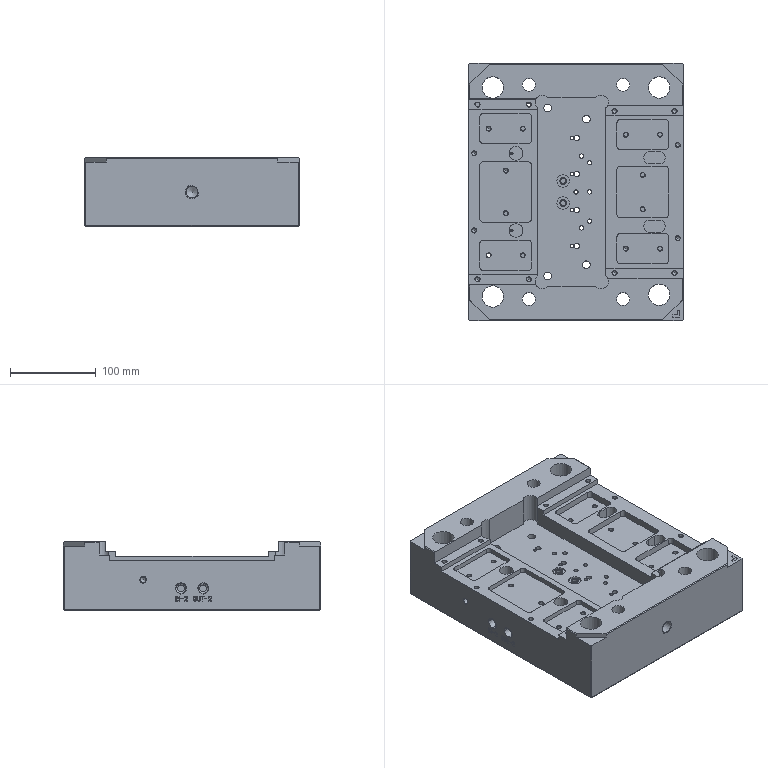NC program | PowerMill | posted with a generic post | part box 250 x 300 x 80 mm
Whole program:
%
O0001
N104 ( POWERMILL CB  : 2026004.0)
N105 ( POST VER      : 2026.0.0.5161)
N106 ( OPTION FILE   : FANUC)
N107 ( OUTPUT WORKPLANE : 2)
N108 (  )
N109 ( TOOL LIST )
N110 (-----------------------------------)
N111 ( NO. | ID    | DIA.| TIP RAD|LENGTH)
N112 (-----------------------------------)
N113 (    1|￠5_2_1| 5.0 |  0.0   |118.24)
N114 (-----------------------------------)
N115 (  )
N116 ( NUMBER OF TOOLPATHS: 1.0 )
N117 ( ESTIMATED PROGRAM DURATION: 0 HOURS 4 MIN 1 SEC)
N118 (  )
N119 G00 G21 G80 G40 G17
N120 G90
N121 G54
N122 G53 Z0.0
N123 (---------------)
N124 ( START TOOLPATH : 34开粗-￠5-钻孔加工 )
N125 (---------------)
N126 ( TOOL NO.    :1 )
N127 ( TOOL TYPE   : DRILL)
N128 ( TOOL ID     : ￠5_2_1)
N129 ( TOOL DIA    : 5.0 LENGTH 118.24)
N130 T1
N131 M6
N132 S700 M03
N133 G00 G90 X20.0 Y-78.0
N134 G43 Z20.0 H1
N135
N136 G05 P0
N137 Z-19.0
N138 G01 Z-27.0 F80.0
N139 G00 Z-19.0
N140 Z-26.4
N141 G01 Z-30.0
N142 G00 Z-19.0
N143 Z-29.4
N144 G01 Z-33.0
N145 G00 Z-19.0
N146 Z-32.4
N147 G01 Z-36.0
N148 G00 Z-19.0
N149 Z-35.4
N150 G01 Z-39.0
N151 G00 Z-19.0
N152 Z-38.4
N153 G01 Z-40.495
N154 G00 Z20.0
N155 X-20.0
N156 Z-19.0
N157 G01 Z-27.0
N158 G00 Z-19.0
N159 Z-26.4
N160 G01 Z-30.0
N161 G00 Z-19.0
N162 Z-29.4
N163 G01 Z-33.0
N164 G00 Z-19.0
N165 Z-32.4
N166 G01 Z-36.0
N167 G00 Z-19.0
N168 Z-35.4
N169 G01 Z-39.0
N170 G00 Z-19.0
N171 Z-38.4
N172 G01 Z-40.495
N173 G00 Z20.0
N174 X-54.1388 Y-119.0
N175 Z-11.2
N176 G01 Z-19.2
N177 G00 Z-11.2
N178 Z-18.6
N179 G01 Z-22.2
N180 G00 Z-11.2
N181 Z-21.6
N182 G01 Z-25.2
N183 G00 Z-11.2
N184 Z-24.6
N185 G01 Z-28.2
N186 G00 Z-11.2
N187 Z-27.6
N188 G01 Z-31.2
N189 G00 Z-11.2
N190 Z-30.6
N191 G01 Z-32.995
N192 G00 Z20.0
N193 X-94.5 Y-115.0
N194 Z-5.0
N195 G01 Z-13.0
N196 G00 Z-5.0
N197 Z-12.4
N198 G01 Z-16.0
N199 G00 Z-5.0
N200 Z-15.4
N201 G01 Z-19.0
N202 G00 Z-5.0
N203 Z-18.4
N204 G01 Z-22.0
N205 G00 Z-5.0
N206 Z-21.4
N207 G01 Z-25.0
N208 G00 Z-5.0
N209 Z-24.4
N210 G01 Z-26.995
N211 G00 Z20.0
N212 X-66.1388 Y-98.0
N213 Z-19.0
N214 G01 Z-27.0
N215 G00 Z-19.0
N216 Z-26.4
N217 G01 Z-30.0
N218 G00 Z-19.0
N219 Z-29.4
N220 G01 Z-33.0
N221 G00 Z-19.0
N222 Z-32.4
N223 G01 Z-36.0
N224 G00 Z-19.0
N225 Z-35.4
N226 G01 Z-39.0
N227 G00 Z-19.0
N228 Z-38.4
N229 G01 Z-40.495
N230 G00 Z20.0
N231 Y-58.0
N232 Z-19.0
N233 G01 Z-27.0
N234 G00 Z-19.0
N235 Z-26.4
N236 G01 Z-30.0
N237 G00 Z-19.0
N238 Z-29.4
N239 G01 Z-33.0
N240 G00 Z-19.0
N241 Z-32.4
N242 G01 Z-36.0
N243 G00 Z-19.0
N244 Z-35.4
N245 G01 Z-39.0
N246 G00 Z-19.0
N247 Z-38.4
N248 G01 Z-40.495
N249 G00 Z20.0
N250 X-94.5 Y-45.0
N251 Z-5.0
N252 G01 Z-13.0
N253 G00 Z-5.0
N254 Z-12.4
N255 G01 Z-16.0
N256 G00 Z-5.0
N257 Z-15.4
N258 G01 Z-19.0
N259 G00 Z-5.0
N260 Z-18.4
N261 G01 Z-22.0
N262 G00 Z-5.0
N263 Z-21.4
N264 G01 Z-25.0
N265 G00 Z-5.0
N266 Z-24.4
N267 G01 Z-26.995
N268 G00 Z20.0
N269 X94.5
N270 Z-5.0
N271 G01 Z-13.0
N272 G00 Z-5.0
N273 Z-12.4
N274 G01 Z-16.0
N275 G00 Z-5.0
N276 Z-15.4
N277 G01 Z-19.0
N278 G00 Z-5.0
N279 Z-18.4
N280 G01 Z-22.0
N281 G00 Z-5.0
N282 Z-21.4
N283 G01 Z-25.0
N284 G00 Z-5.0
N285 Z-24.4
N286 G01 Z-26.995
N287 G00 Z20.0
N288 X67.0 Y-58.0
N289 Z-19.0
N290 G01 Z-27.0
N291 G00 Z-19.0
N292 Z-26.4
N293 G01 Z-30.0
N294 G00 Z-19.0
N295 Z-29.4
N296 G01 Z-33.0
N297 G00 Z-19.0
N298 Z-32.4
N299 G01 Z-36.0
N300 G00 Z-19.0
N301 Z-35.4
N302 G01 Z-39.0
N303 G00 Z-19.0
N304 Z-38.4
N305 G01 Z-40.495
N306 G00 Z20.0
N307 Y-98.0
N308 Z-19.0
N309 G01 Z-27.0
N310 G00 Z-19.0
N311 Z-26.4
N312 G01 Z-30.0
N313 G00 Z-19.0
N314 Z-29.4
N315 G01 Z-33.0
N316 G00 Z-19.0
N317 Z-32.4
N318 G01 Z-36.0
N319 G00 Z-19.0
N320 Z-35.4
N321 G01 Z-39.0
N322 G00 Z-19.0
N323 Z-38.4
N324 G01 Z-40.495
N325 G00 Z20.0
N326 X55.0 Y-119.0
N327 Z-11.2
N328 G01 Z-19.2
N329 G00 Z-11.2
N330 Z-18.6
N331 G01 Z-22.2
N332 G00 Z-11.2
N333 Z-21.6
N334 G01 Z-25.2
N335 G00 Z-11.2
N336 Z-24.6
N337 G01 Z-28.2
N338 G00 Z-11.2
N339 Z-27.6
N340 G01 Z-31.2
N341 G00 Z-11.2
N342 Z-30.6
N343 G01 Z-32.995
N344 G00 Z20.0
N345 X94.5 Y-115.0
N346 Z-5.0
N347 G01 Z-13.0
N348 G00 Z-5.0
N349 Z-12.4
N350 G01 Z-16.0
N351 G00 Z-5.0
N352 Z-15.4
N353 G01 Z-19.0
N354 G00 Z-5.0
N355 Z-18.4
N356 G01 Z-22.0
N357 G00 Z-5.0
N358 Z-21.4
N359 G01 Z-25.0
N360 G00 Z-5.0
N361 Z-24.4
N362 G01 Z-26.995
N363 G00 Z20.0
N364 G05 P0
N365 (---------------)
N366 ( END TOOLPATH : 34开粗-￠5-钻孔加工 )
N367 (---------------)
N368
N369 M05
N370 G53 Z0.0
N371 M30
%